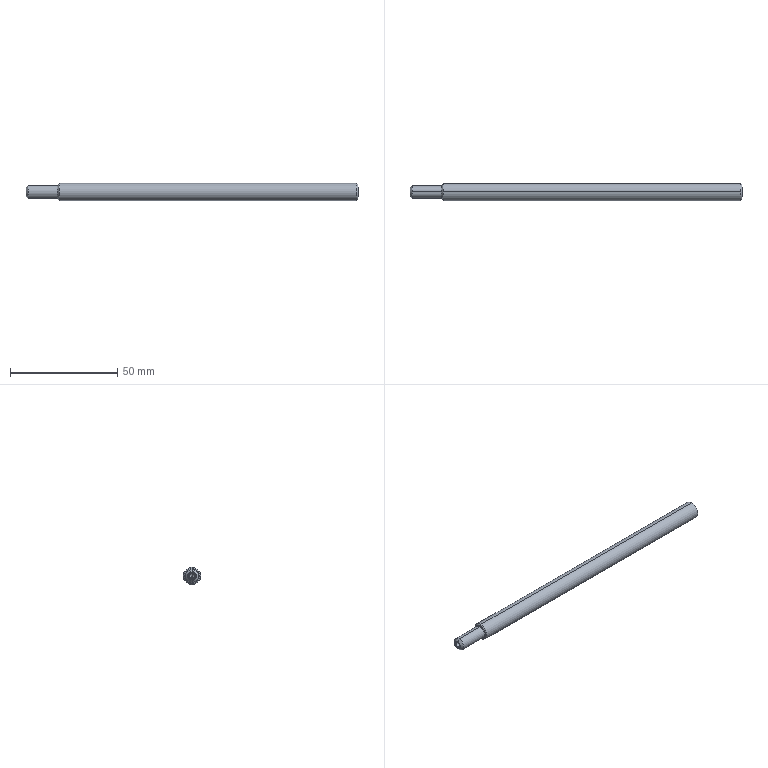Part | SolidWorks | features BaseBody 1, MoveFace 1 | 1 solid | 27 faces | box 155 x 8 x 8 mm | volume 7283 mm3 | cone 14 | cylinder 8 | plane 3 | spline 2 | commonest cylinder face diameters 2.459 x2 3.242 x2 6 x2 8 x2
STEP:
#1=CARTESIAN_POINT('',(-15.3,0.,3.));
#2=VERTEX_POINT('',#1);
#3=CARTESIAN_POINT('',(-15.3,0.,-3.));
#4=VERTEX_POINT('',#3);
#5=CARTESIAN_POINT('',(-15.3,0.,0.));
#6=DIRECTION('',(-1.,0.,0.));
#7=DIRECTION('',(0.,0.,-1.));
#8=AXIS2_PLACEMENT_3D('',#5,#6,#7);
#9=CIRCLE('',#8,3.);
#10=EDGE_CURVE('',#2,#4,#9,.T.);
#11=ORIENTED_EDGE('',*,*,#10,.F.);
#12=CARTESIAN_POINT('',(-15.,0.,3.3));
#13=VERTEX_POINT('',#12);
#14=CARTESIAN_POINT('',(-15.3,0.,3.3));
#15=DIRECTION('',(0.,-1.,0.));
#16=DIRECTION('',(0.,0.,1.));
#17=AXIS2_PLACEMENT_3D('',#14,#15,#16);
#18=CIRCLE('',#17,0.3);
#19=EDGE_CURVE('',#2,#13,#18,.T.);
#20=ORIENTED_EDGE('',*,*,#19,.T.);
#21=CARTESIAN_POINT('',(-15.,0.,-3.3));
#22=VERTEX_POINT('',#21);
#23=CARTESIAN_POINT('',(-15.,0.,3.3));
#24=CARTESIAN_POINT('',(-15.,6.6,3.3));
#25=CARTESIAN_POINT('',(-15.,6.6,-3.3));
#26=CARTESIAN_POINT('',(-15.,0.,-3.3));
#27=(BOUNDED_CURVE()B_SPLINE_CURVE(3,(#23,#24,#25,#26),.UNSPECIFIED.,.F.,.F.)B_SPLINE_CURVE_WITH_KNOTS((4,4),(0.5,1.),.UNSPECIFIED.)CURVE()GEOMETRIC_REPRESENTATION_ITEM()RATIONAL_B_SPLINE_CURVE((1.,0.3333,0.3333,1.))REPRESENTATION_ITEM(''));
#28=EDGE_CURVE('',#13,#22,#27,.T.);
#29=ORIENTED_EDGE('',*,*,#28,.T.);
#30=CARTESIAN_POINT('',(-15.3,0.,-3.3));
#31=DIRECTION('',(0.,1.,0.));
#32=DIRECTION('',(0.,0.,-1.));
#33=AXIS2_PLACEMENT_3D('',#30,#31,#32);
#34=CIRCLE('',#33,0.3);
#35=EDGE_CURVE('',#4,#22,#34,.T.);
#36=ORIENTED_EDGE('',*,*,#35,.F.);
#37=EDGE_LOOP('',(#11,#20,#29,#36));
#38=FACE_OUTER_BOUND('',#37,.T.);
#39=CARTESIAN_POINT('',(-15.3,0.,-3.));
#40=CARTESIAN_POINT('',(-15.3,6.,-3.));
#41=CARTESIAN_POINT('',(-15.3,6.,3.));
#42=CARTESIAN_POINT('',(-15.3,0.,3.));
#43=CARTESIAN_POINT('',(-15.124,0.,-3.));
#44=CARTESIAN_POINT('',(-15.124,6.,-3.));
#45=CARTESIAN_POINT('',(-15.124,6.,3.));
#46=CARTESIAN_POINT('',(-15.124,0.,3.));
#47=CARTESIAN_POINT('',(-15.,0.,-3.124));
#48=CARTESIAN_POINT('',(-15.,6.249,-3.124));
#49=CARTESIAN_POINT('',(-15.,6.249,3.124));
#50=CARTESIAN_POINT('',(-15.,0.,3.124));
#51=CARTESIAN_POINT('',(-15.,0.,-3.3));
#52=CARTESIAN_POINT('',(-15.,6.6,-3.3));
#53=CARTESIAN_POINT('',(-15.,6.6,3.3));
#54=CARTESIAN_POINT('',(-15.,0.,3.3));
#55=(BOUNDED_SURFACE()B_SPLINE_SURFACE(3,3,((#39,#40,#41,#42),(#43,#44,#45,#46),(#47,#48,#49,#50),(#51,#52,#53,#54)),.UNSPECIFIED.,.F.,.F.,.F.)B_SPLINE_SURFACE_WITH_KNOTS((4,4),(4,4),(0.,1.),(0.,1.),.UNSPECIFIED.)GEOMETRIC_REPRESENTATION_ITEM()RATIONAL_B_SPLINE_SURFACE(((1.,0.3333,0.3333,1.),(0.8047,0.2682,0.2682,0.8047),(0.8047,0.2682,0.2682,0.8047),(1.,0.3333,0.3333,1.)))REPRESENTATION_ITEM('')SURFACE());
#56=ADVANCED_FACE('',(#38),#55,.F.);
#57=CARTESIAN_POINT('',(124.5,0.,4.));
#58=VERTEX_POINT('',#57);
#59=CARTESIAN_POINT('',(124.5,0.,-4.));
#60=VERTEX_POINT('',#59);
#61=CARTESIAN_POINT('',(124.5,0.,0.));
#62=DIRECTION('',(-1.,0.,0.));
#63=DIRECTION('',(0.,0.,1.));
#64=AXIS2_PLACEMENT_3D('',#61,#62,#63);
#65=CIRCLE('',#64,4.);
#66=EDGE_CURVE('',#58,#60,#65,.T.);
#67=ORIENTED_EDGE('',*,*,#66,.T.);
#68=CARTESIAN_POINT('',(-14.5,0.,-4.));
#69=VERTEX_POINT('',#68);
#70=CARTESIAN_POINT('',(110.,0.,-4.));
#71=DIRECTION('',(-1.,0.,0.));
#72=VECTOR('',#71,1000.);
#73=LINE('',#70,#72);
#74=EDGE_CURVE('',#60,#69,#73,.T.);
#75=ORIENTED_EDGE('',*,*,#74,.T.);
#76=CARTESIAN_POINT('',(-14.5,0.,4.));
#77=VERTEX_POINT('',#76);
#78=CARTESIAN_POINT('',(-14.5,0.,0.));
#79=DIRECTION('',(1.,0.,0.));
#80=DIRECTION('',(0.,0.,1.));
#81=AXIS2_PLACEMENT_3D('',#78,#79,#80);
#82=CIRCLE('',#81,4.);
#83=EDGE_CURVE('',#69,#77,#82,.T.);
#84=ORIENTED_EDGE('',*,*,#83,.T.);
#85=CARTESIAN_POINT('',(110.,0.,4.));
#86=DIRECTION('',(-1.,0.,0.));
#87=VECTOR('',#86,1000.);
#88=LINE('',#85,#87);
#89=EDGE_CURVE('',#58,#77,#88,.T.);
#90=ORIENTED_EDGE('',*,*,#89,.F.);
#91=EDGE_LOOP('',(#67,#75,#84,#90));
#92=FACE_OUTER_BOUND('',#91,.T.);
#93=CARTESIAN_POINT('',(110.,0.,0.));
#94=DIRECTION('',(-1.,0.,0.));
#95=DIRECTION('',(0.,0.,1.));
#96=AXIS2_PLACEMENT_3D('',#93,#94,#95);
#97=CYLINDRICAL_SURFACE('',#96,4.);
#98=ADVANCED_FACE('',(#92),#97,.T.);
#99=CARTESIAN_POINT('',(-15.,0.,-3.5));
#100=VERTEX_POINT('',#99);
#101=CARTESIAN_POINT('',(-15.,0.,3.5));
#102=VERTEX_POINT('',#101);
#103=CARTESIAN_POINT('',(-15.,0.,0.));
#104=DIRECTION('',(1.,0.,0.));
#105=DIRECTION('',(0.,0.,-1.));
#106=AXIS2_PLACEMENT_3D('',#103,#104,#105);
#107=CIRCLE('',#106,3.5);
#108=EDGE_CURVE('',#100,#102,#107,.T.);
#109=ORIENTED_EDGE('',*,*,#108,.T.);
#110=CARTESIAN_POINT('',(-14.5,0.,4.));
#111=DIRECTION('',(0.7071,0.,0.7071));
#112=VECTOR('',#111,1000.);
#113=LINE('',#110,#112);
#114=EDGE_CURVE('',#102,#77,#113,.T.);
#115=ORIENTED_EDGE('',*,*,#114,.T.);
#116=ORIENTED_EDGE('',*,*,#83,.F.);
#117=CARTESIAN_POINT('',(-14.5,0.,-4.));
#118=DIRECTION('',(0.7071,0.,-0.7071));
#119=VECTOR('',#118,1000.);
#120=LINE('',#117,#119);
#121=EDGE_CURVE('',#100,#69,#120,.T.);
#122=ORIENTED_EDGE('',*,*,#121,.F.);
#123=EDGE_LOOP('',(#109,#115,#116,#122));
#124=FACE_OUTER_BOUND('',#123,.T.);
#125=CARTESIAN_POINT('',(-14.5,0.,0.));
#126=DIRECTION('',(1.,0.,0.));
#127=DIRECTION('',(0.,0.,-1.));
#128=AXIS2_PLACEMENT_3D('',#125,#126,#127);
#129=CONICAL_SURFACE('',#128,4.,0.7854);
#130=ADVANCED_FACE('',(#124),#129,.T.);
#131=CARTESIAN_POINT('',(125.,0.,3.5));
#132=VERTEX_POINT('',#131);
#133=CARTESIAN_POINT('',(125.,0.,-3.5));
#134=VERTEX_POINT('',#133);
#135=CARTESIAN_POINT('',(125.,0.,0.));
#136=DIRECTION('',(-1.,0.,0.));
#137=DIRECTION('',(0.,0.,1.));
#138=AXIS2_PLACEMENT_3D('',#135,#136,#137);
#139=CIRCLE('',#138,3.5);
#140=EDGE_CURVE('',#132,#134,#139,.T.);
#141=ORIENTED_EDGE('',*,*,#140,.T.);
#142=CARTESIAN_POINT('',(124.5,0.,-4.));
#143=DIRECTION('',(-0.7071,0.,-0.7071));
#144=VECTOR('',#143,1000.);
#145=LINE('',#142,#144);
#146=EDGE_CURVE('',#134,#60,#145,.T.);
#147=ORIENTED_EDGE('',*,*,#146,.T.);
#148=ORIENTED_EDGE('',*,*,#66,.F.);
#149=CARTESIAN_POINT('',(124.5,0.,4.));
#150=DIRECTION('',(-0.7071,0.,0.7071));
#151=VECTOR('',#150,1000.);
#152=LINE('',#149,#151);
#153=EDGE_CURVE('',#132,#58,#152,.T.);
#154=ORIENTED_EDGE('',*,*,#153,.F.);
#155=EDGE_LOOP('',(#141,#147,#148,#154));
#156=FACE_OUTER_BOUND('',#155,.T.);
#157=CARTESIAN_POINT('',(124.5,0.,0.));
#158=DIRECTION('',(-1.,0.,0.));
#159=DIRECTION('',(0.,0.,1.));
#160=AXIS2_PLACEMENT_3D('',#157,#158,#159);
#161=CONICAL_SURFACE('',#160,4.,0.7854);
#162=ADVANCED_FACE('',(#156),#161,.T.);
#163=CARTESIAN_POINT('',(124.621,0.,1.621));
#164=VERTEX_POINT('',#163);
#165=CARTESIAN_POINT('',(124.621,0.,-1.621));
#166=VERTEX_POINT('',#165);
#167=CARTESIAN_POINT('',(124.621,0.,0.));
#168=DIRECTION('',(1.,0.,0.));
#169=DIRECTION('',(0.,0.,-1.));
#170=AXIS2_PLACEMENT_3D('',#167,#168,#169);
#171=CIRCLE('',#170,1.621);
#172=EDGE_CURVE('',#164,#166,#171,.T.);
#173=ORIENTED_EDGE('',*,*,#172,.F.);
#174=CARTESIAN_POINT('',(125.,0.,2.));
#175=VERTEX_POINT('',#174);
#176=CARTESIAN_POINT('',(125.,0.,2.));
#177=DIRECTION('',(0.7071,0.,0.7071));
#178=VECTOR('',#177,1000.);
#179=LINE('',#176,#178);
#180=EDGE_CURVE('',#164,#175,#179,.T.);
#181=ORIENTED_EDGE('',*,*,#180,.T.);
#182=CARTESIAN_POINT('',(125.,0.,-2.));
#183=VERTEX_POINT('',#182);
#184=CARTESIAN_POINT('',(125.,0.,0.));
#185=DIRECTION('',(1.,0.,0.));
#186=DIRECTION('',(0.,0.,-1.));
#187=AXIS2_PLACEMENT_3D('',#184,#185,#186);
#188=CIRCLE('',#187,2.);
#189=EDGE_CURVE('',#175,#183,#188,.T.);
#190=ORIENTED_EDGE('',*,*,#189,.T.);
#191=CARTESIAN_POINT('',(125.,0.,-2.));
#192=DIRECTION('',(0.7071,0.,-0.7071));
#193=VECTOR('',#192,1000.);
#194=LINE('',#191,#193);
#195=EDGE_CURVE('',#166,#183,#194,.T.);
#196=ORIENTED_EDGE('',*,*,#195,.F.);
#197=EDGE_LOOP('',(#173,#181,#190,#196));
#198=FACE_OUTER_BOUND('',#197,.T.);
#199=CARTESIAN_POINT('',(125.,0.,0.));
#200=DIRECTION('',(1.,0.,0.));
#201=DIRECTION('',(0.,0.,-1.));
#202=AXIS2_PLACEMENT_3D('',#199,#200,#201);
#203=CONICAL_SURFACE('',#202,2.,0.7854);
#204=ADVANCED_FACE('',(#198),#203,.F.);
#205=ORIENTED_EDGE('',*,*,#10,.T.);
#206=CARTESIAN_POINT('',(-29.,0.,-3.));
#207=VERTEX_POINT('',#206);
#208=CARTESIAN_POINT('',(110.,0.,-3.));
#209=DIRECTION('',(-1.,0.,0.));
#210=VECTOR('',#209,1000.);
#211=LINE('',#208,#210);
#212=EDGE_CURVE('',#4,#207,#211,.T.);
#213=ORIENTED_EDGE('',*,*,#212,.T.);
#214=CARTESIAN_POINT('',(-29.,0.,3.));
#215=VERTEX_POINT('',#214);
#216=CARTESIAN_POINT('',(-29.,0.,0.));
#217=DIRECTION('',(1.,0.,0.));
#218=DIRECTION('',(0.,0.,1.));
#219=AXIS2_PLACEMENT_3D('',#216,#217,#218);
#220=CIRCLE('',#219,3.);
#221=EDGE_CURVE('',#207,#215,#220,.T.);
#222=ORIENTED_EDGE('',*,*,#221,.T.);
#223=CARTESIAN_POINT('',(110.,0.,3.));
#224=DIRECTION('',(-1.,0.,0.));
#225=VECTOR('',#224,1000.);
#226=LINE('',#223,#225);
#227=EDGE_CURVE('',#2,#215,#226,.T.);
#228=ORIENTED_EDGE('',*,*,#227,.F.);
#229=EDGE_LOOP('',(#205,#213,#222,#228));
#230=FACE_OUTER_BOUND('',#229,.T.);
#231=CARTESIAN_POINT('',(110.,0.,0.));
#232=DIRECTION('',(-1.,0.,0.));
#233=DIRECTION('',(0.,0.,1.));
#234=AXIS2_PLACEMENT_3D('',#231,#232,#233);
#235=CYLINDRICAL_SURFACE('',#234,3.);
#236=ADVANCED_FACE('',(#230),#235,.T.);
#237=ORIENTED_EDGE('',*,*,#172,.T.);
#238=CARTESIAN_POINT('',(111.936,0.,-1.621));
#239=VERTEX_POINT('',#238);
#240=CARTESIAN_POINT('',(125.,0.,-1.621));
#241=DIRECTION('',(-1.,0.,0.));
#242=VECTOR('',#241,1000.);
#243=LINE('',#240,#242);
#244=EDGE_CURVE('',#166,#239,#243,.T.);
#245=ORIENTED_EDGE('',*,*,#244,.T.);
#246=CARTESIAN_POINT('',(111.936,0.,1.621));
#247=VERTEX_POINT('',#246);
#248=CARTESIAN_POINT('',(111.936,0.,0.));
#249=DIRECTION('',(1.,0.,0.));
#250=DIRECTION('',(0.,0.,1.));
#251=AXIS2_PLACEMENT_3D('',#248,#249,#250);
#252=CIRCLE('',#251,1.621);
#253=EDGE_CURVE('',#247,#239,#252,.T.);
#254=ORIENTED_EDGE('',*,*,#253,.F.);
#255=CARTESIAN_POINT('',(125.,0.,1.621));
#256=DIRECTION('',(-1.,0.,0.));
#257=VECTOR('',#256,1000.);
#258=LINE('',#255,#257);
#259=EDGE_CURVE('',#164,#247,#258,.T.);
#260=ORIENTED_EDGE('',*,*,#259,.F.);
#261=EDGE_LOOP('',(#237,#245,#254,#260));
#262=FACE_OUTER_BOUND('',#261,.T.);
#263=CARTESIAN_POINT('',(125.,0.,0.));
#264=DIRECTION('',(-1.,0.,0.));
#265=DIRECTION('',(0.,0.,1.));
#266=AXIS2_PLACEMENT_3D('',#263,#264,#265);
#267=CYLINDRICAL_SURFACE('',#266,1.621);
#268=ADVANCED_FACE('',(#262),#267,.F.);
#269=CARTESIAN_POINT('',(-30.,0.,-2.));
#270=VERTEX_POINT('',#269);
#271=CARTESIAN_POINT('',(-30.,0.,2.));
#272=VERTEX_POINT('',#271);
#273=CARTESIAN_POINT('',(-30.,0.,0.));
#274=DIRECTION('',(1.,0.,0.));
#275=DIRECTION('',(0.,0.,-1.));
#276=AXIS2_PLACEMENT_3D('',#273,#274,#275);
#277=CIRCLE('',#276,2.);
#278=EDGE_CURVE('',#270,#272,#277,.T.);
#279=ORIENTED_EDGE('',*,*,#278,.T.);
#280=CARTESIAN_POINT('',(-29.,0.,3.));
#281=DIRECTION('',(0.7071,0.,0.7071));
#282=VECTOR('',#281,1000.);
#283=LINE('',#280,#282);
#284=EDGE_CURVE('',#272,#215,#283,.T.);
#285=ORIENTED_EDGE('',*,*,#284,.T.);
#286=ORIENTED_EDGE('',*,*,#221,.F.);
#287=CARTESIAN_POINT('',(-29.,0.,-3.));
#288=DIRECTION('',(0.7071,0.,-0.7071));
#289=VECTOR('',#288,1000.);
#290=LINE('',#287,#289);
#291=EDGE_CURVE('',#270,#207,#290,.T.);
#292=ORIENTED_EDGE('',*,*,#291,.F.);
#293=EDGE_LOOP('',(#279,#285,#286,#292));
#294=FACE_OUTER_BOUND('',#293,.T.);
#295=CARTESIAN_POINT('',(-29.,0.,0.));
#296=DIRECTION('',(1.,0.,0.));
#297=DIRECTION('',(0.,0.,-1.));
#298=AXIS2_PLACEMENT_3D('',#295,#296,#297);
#299=CONICAL_SURFACE('',#298,3.,0.7854);
#300=ADVANCED_FACE('',(#294),#299,.T.);
#301=CARTESIAN_POINT('',(111.,0.,0.));
#302=VERTEX_POINT('',#301);
#303=CARTESIAN_POINT('',(111.936,0.,-1.621));
#304=DIRECTION('',(0.5,0.,-0.866));
#305=VECTOR('',#304,1000.);
#306=LINE('',#303,#305);
#307=EDGE_CURVE('',#302,#239,#306,.T.);
#308=ORIENTED_EDGE('',*,*,#307,.F.);
#309=CARTESIAN_POINT('',(111.936,0.,1.621));
#310=DIRECTION('',(0.5,0.,0.866));
#311=VECTOR('',#310,1000.);
#312=LINE('',#309,#311);
#313=EDGE_CURVE('',#302,#247,#312,.T.);
#314=ORIENTED_EDGE('',*,*,#313,.T.);
#315=ORIENTED_EDGE('',*,*,#253,.T.);
#316=EDGE_LOOP('',(#308,#314,#315));
#317=FACE_OUTER_BOUND('',#316,.T.);
#318=CARTESIAN_POINT('',(111.936,0.,0.));
#319=DIRECTION('',(1.,0.,0.));
#320=DIRECTION('',(0.,0.,-1.));
#321=AXIS2_PLACEMENT_3D('',#318,#319,#320);
#322=CONICAL_SURFACE('',#321,1.621,1.047);
#323=ADVANCED_FACE('',(#317),#322,.F.);
#324=CARTESIAN_POINT('',(-29.729,0.,-1.23));
#325=VERTEX_POINT('',#324);
#326=CARTESIAN_POINT('',(-29.729,0.,1.23));
#327=VERTEX_POINT('',#326);
#328=CARTESIAN_POINT('',(-29.729,0.,0.));
#329=DIRECTION('',(-1.,0.,0.));
#330=DIRECTION('',(0.,0.,1.));
#331=AXIS2_PLACEMENT_3D('',#328,#329,#330);
#332=CIRCLE('',#331,1.23);
#333=EDGE_CURVE('',#325,#327,#332,.T.);
#334=ORIENTED_EDGE('',*,*,#333,.F.);
#335=CARTESIAN_POINT('',(-30.,0.,-1.5));
#336=VERTEX_POINT('',#335);
#337=CARTESIAN_POINT('',(-30.,0.,-1.5));
#338=DIRECTION('',(-0.7071,0.,-0.7071));
#339=VECTOR('',#338,1000.);
#340=LINE('',#337,#339);
#341=EDGE_CURVE('',#325,#336,#340,.T.);
#342=ORIENTED_EDGE('',*,*,#341,.T.);
#343=CARTESIAN_POINT('',(-30.,0.,1.5));
#344=VERTEX_POINT('',#343);
#345=CARTESIAN_POINT('',(-30.,0.,0.));
#346=DIRECTION('',(-1.,0.,0.));
#347=DIRECTION('',(0.,0.,1.));
#348=AXIS2_PLACEMENT_3D('',#345,#346,#347);
#349=CIRCLE('',#348,1.5);
#350=EDGE_CURVE('',#336,#344,#349,.T.);
#351=ORIENTED_EDGE('',*,*,#350,.T.);
#352=CARTESIAN_POINT('',(-30.,0.,1.5));
#353=DIRECTION('',(-0.7071,0.,0.7071));
#354=VECTOR('',#353,1000.);
#355=LINE('',#352,#354);
#356=EDGE_CURVE('',#327,#344,#355,.T.);
#357=ORIENTED_EDGE('',*,*,#356,.F.);
#358=EDGE_LOOP('',(#334,#342,#351,#357));
#359=FACE_OUTER_BOUND('',#358,.T.);
#360=CARTESIAN_POINT('',(-30.,0.,0.));
#361=DIRECTION('',(-1.,0.,0.));
#362=DIRECTION('',(0.,0.,1.));
#363=AXIS2_PLACEMENT_3D('',#360,#361,#362);
#364=CONICAL_SURFACE('',#363,1.5,0.7854);
#365=ADVANCED_FACE('',(#359),#364,.F.);
#366=CARTESIAN_POINT('',(-19.21,0.,-1.23));
#367=VERTEX_POINT('',#366);
#368=CARTESIAN_POINT('',(-19.21,0.,1.23));
#369=VERTEX_POINT('',#368);
#370=CARTESIAN_POINT('',(-19.21,0.,0.));
#371=DIRECTION('',(-1.,0.,0.));
#372=DIRECTION('',(0.,0.,1.));
#373=AXIS2_PLACEMENT_3D('',#370,#371,#372);
#374=CIRCLE('',#373,1.23);
#375=EDGE_CURVE('',#367,#369,#374,.T.);
#376=ORIENTED_EDGE('',*,*,#375,.F.);
#377=CARTESIAN_POINT('',(-18.5,0.,-1.23));
#378=DIRECTION('',(-1.,0.,0.));
#379=VECTOR('',#378,1000.);
#380=LINE('',#377,#379);
#381=EDGE_CURVE('',#367,#325,#380,.T.);
#382=ORIENTED_EDGE('',*,*,#381,.T.);
#383=ORIENTED_EDGE('',*,*,#333,.T.);
#384=CARTESIAN_POINT('',(-18.5,0.,1.23));
#385=DIRECTION('',(-1.,0.,0.));
#386=VECTOR('',#385,1000.);
#387=LINE('',#384,#386);
#388=EDGE_CURVE('',#369,#327,#387,.T.);
#389=ORIENTED_EDGE('',*,*,#388,.F.);
#390=EDGE_LOOP('',(#376,#382,#383,#389));
#391=FACE_OUTER_BOUND('',#390,.T.);
#392=CARTESIAN_POINT('',(-18.5,0.,0.));
#393=DIRECTION('',(-1.,0.,0.));
#394=DIRECTION('',(0.,0.,1.));
#395=AXIS2_PLACEMENT_3D('',#392,#393,#394);
#396=CYLINDRICAL_SURFACE('',#395,1.23);
#397=ADVANCED_FACE('',(#391),#396,.F.);
#398=CARTESIAN_POINT('',(-18.5,0.,0.));
#399=VERTEX_POINT('',#398);
#400=CARTESIAN_POINT('',(-19.21,0.,1.23));
#401=DIRECTION('',(-0.5,0.,0.866));
#402=VECTOR('',#401,1000.);
#403=LINE('',#400,#402);
#404=EDGE_CURVE('',#399,#369,#403,.T.);
#405=ORIENTED_EDGE('',*,*,#404,.F.);
#406=CARTESIAN_POINT('',(-19.21,0.,-1.23));
#407=DIRECTION('',(-0.5,0.,-0.866));
#408=VECTOR('',#407,1000.);
#409=LINE('',#406,#408);
#410=EDGE_CURVE('',#399,#367,#409,.T.);
#411=ORIENTED_EDGE('',*,*,#410,.T.);
#412=ORIENTED_EDGE('',*,*,#375,.T.);
#413=EDGE_LOOP('',(#405,#411,#412));
#414=FACE_OUTER_BOUND('',#413,.T.);
#415=CARTESIAN_POINT('',(-19.21,0.,0.));
#416=DIRECTION('',(-1.,0.,0.));
#417=DIRECTION('',(0.,0.,1.));
#418=AXIS2_PLACEMENT_3D('',#415,#416,#417);
#419=CONICAL_SURFACE('',#418,1.23,1.047);
#420=ADVANCED_FACE('',(#414),#419,.F.);
#421=ORIENTED_EDGE('',*,*,#74,.F.);
#422=CARTESIAN_POINT('',(124.5,0.,0.));
#423=DIRECTION('',(-1.,0.,0.));
#424=DIRECTION('',(0.,0.,1.));
#425=AXIS2_PLACEMENT_3D('',#422,#423,#424);
#426=CIRCLE('',#425,4.);
#427=EDGE_CURVE('',#60,#58,#426,.T.);
#428=ORIENTED_EDGE('',*,*,#427,.T.);
#429=ORIENTED_EDGE('',*,*,#89,.T.);
#430=CARTESIAN_POINT('',(-14.5,0.,0.));
#431=DIRECTION('',(1.,0.,0.));
#432=DIRECTION('',(0.,0.,1.));
#433=AXIS2_PLACEMENT_3D('',#430,#431,#432);
#434=CIRCLE('',#433,4.);
#435=EDGE_CURVE('',#77,#69,#434,.T.);
#436=ORIENTED_EDGE('',*,*,#435,.T.);
#437=EDGE_LOOP('',(#421,#428,#429,#436));
#438=FACE_OUTER_BOUND('',#437,.T.);
#439=CARTESIAN_POINT('',(110.,0.,0.));
#440=DIRECTION('',(-1.,0.,0.));
#441=DIRECTION('',(0.,0.,1.));
#442=AXIS2_PLACEMENT_3D('',#439,#440,#441);
#443=CYLINDRICAL_SURFACE('',#442,4.);
#444=ADVANCED_FACE('',(#438),#443,.T.);
#445=ORIENTED_EDGE('',*,*,#114,.F.);
#446=CARTESIAN_POINT('',(-15.,0.,0.));
#447=DIRECTION('',(1.,0.,0.));
#448=DIRECTION('',(0.,0.,-1.));
#449=AXIS2_PLACEMENT_3D('',#446,#447,#448);
#450=CIRCLE('',#449,3.5);
#451=EDGE_CURVE('',#102,#100,#450,.T.);
#452=ORIENTED_EDGE('',*,*,#451,.T.);
#453=ORIENTED_EDGE('',*,*,#121,.T.);
#454=ORIENTED_EDGE('',*,*,#435,.F.);
#455=EDGE_LOOP('',(#445,#452,#453,#454));
#456=FACE_OUTER_BOUND('',#455,.T.);
#457=CARTESIAN_POINT('',(-14.5,0.,0.));
#458=DIRECTION('',(1.,0.,0.));
#459=DIRECTION('',(0.,0.,-1.));
#460=AXIS2_PLACEMENT_3D('',#457,#458,#459);
#461=CONICAL_SURFACE('',#460,4.,0.7854);
#462=ADVANCED_FACE('',(#456),#461,.T.);
#463=ORIENTED_EDGE('',*,*,#146,.F.);
#464=CARTESIAN_POINT('',(125.,0.,0.));
#465=DIRECTION('',(-1.,0.,0.));
#466=DIRECTION('',(0.,0.,1.));
#467=AXIS2_PLACEMENT_3D('',#464,#465,#466);
#468=CIRCLE('',#467,3.5);
#469=EDGE_CURVE('',#134,#132,#468,.T.);
#470=ORIENTED_EDGE('',*,*,#469,.T.);
#471=ORIENTED_EDGE('',*,*,#153,.T.);
#472=ORIENTED_EDGE('',*,*,#427,.F.);
#473=EDGE_LOOP('',(#463,#470,#471,#472));
#474=FACE_OUTER_BOUND('',#473,.T.);
#475=CARTESIAN_POINT('',(124.5,0.,0.));
#476=DIRECTION('',(-1.,0.,0.));
#477=DIRECTION('',(0.,0.,1.));
#478=AXIS2_PLACEMENT_3D('',#475,#476,#477);
#479=CONICAL_SURFACE('',#478,4.,0.7854);
#480=ADVANCED_FACE('',(#474),#479,.T.);
#481=CARTESIAN_POINT('',(-15.,0.,-3.3));
#482=CARTESIAN_POINT('',(-15.,-6.6,-3.3));
#483=CARTESIAN_POINT('',(-15.,-6.6,3.3));
#484=CARTESIAN_POINT('',(-15.,0.,3.3));
#485=(BOUNDED_CURVE()B_SPLINE_CURVE(3,(#481,#482,#483,#484),.UNSPECIFIED.,.F.,.F.)B_SPLINE_CURVE_WITH_KNOTS((4,4),(0.,0.5),.UNSPECIFIED.)CURVE()GEOMETRIC_REPRESENTATION_ITEM()RATIONAL_B_SPLINE_CURVE((1.,0.3333,0.3333,1.))REPRESENTATION_ITEM(''));
#486=EDGE_CURVE('',#22,#13,#485,.T.);
#487=ORIENTED_EDGE('',*,*,#486,.F.);
#488=ORIENTED_EDGE('',*,*,#28,.F.);
#489=EDGE_LOOP('',(#487,#488));
#490=FACE_BOUND('',#489,.T.);
#491=ORIENTED_EDGE('',*,*,#108,.F.);
#492=ORIENTED_EDGE('',*,*,#451,.F.);
#493=EDGE_LOOP('',(#491,#492));
#494=FACE_OUTER_BOUND('',#493,.T.);
#495=CARTESIAN_POINT('',(-15.,3.3,0.));
#496=DIRECTION('',(1.,0.,0.));
#497=DIRECTION('',(0.,0.,-1.));
#498=AXIS2_PLACEMENT_3D('',#495,#496,#497);
#499=PLANE('',#498);
#500=ADVANCED_FACE('',(#490,#494),#499,.F.);
#501=ORIENTED_EDGE('',*,*,#140,.F.);
#502=ORIENTED_EDGE('',*,*,#469,.F.);
#503=EDGE_LOOP('',(#501,#502));
#504=FACE_OUTER_BOUND('',#503,.T.);
#505=CARTESIAN_POINT('',(125.,0.,0.));
#506=DIRECTION('',(1.,0.,0.));
#507=DIRECTION('',(0.,0.,-1.));
#508=AXIS2_PLACEMENT_3D('',#505,#506,#507);
#509=CIRCLE('',#508,2.);
#510=EDGE_CURVE('',#183,#175,#509,.T.);
#511=ORIENTED_EDGE('',*,*,#510,.F.);
#512=ORIENTED_EDGE('',*,*,#189,.F.);
#513=EDGE_LOOP('',(#511,#512));
#514=FACE_BOUND('',#513,.T.);
#515=CARTESIAN_POINT('',(125.,3.5,0.));
#516=DIRECTION('',(-1.,0.,0.));
#517=DIRECTION('',(0.,0.,1.));
#518=AXIS2_PLACEMENT_3D('',#515,#516,#517);
#519=PLANE('',#518);
#520=ADVANCED_FACE('',(#504,#514),#519,.F.);
#521=ORIENTED_EDGE('',*,*,#19,.F.);
#522=CARTESIAN_POINT('',(-15.3,0.,0.));
#523=DIRECTION('',(-1.,0.,0.));
#524=DIRECTION('',(0.,0.,-1.));
#525=AXIS2_PLACEMENT_3D('',#522,#523,#524);
#526=CIRCLE('',#525,3.);
#527=EDGE_CURVE('',#4,#2,#526,.T.);
#528=ORIENTED_EDGE('',*,*,#527,.F.);
#529=ORIENTED_EDGE('',*,*,#35,.T.);
#530=ORIENTED_EDGE('',*,*,#486,.T.);
#531=EDGE_LOOP('',(#521,#528,#529,#530));
#532=FACE_OUTER_BOUND('',#531,.T.);
#533=CARTESIAN_POINT('',(-15.3,0.,3.));
#534=CARTESIAN_POINT('',(-15.3,-6.,3.));
#535=CARTESIAN_POINT('',(-15.3,-6.,-3.));
#536=CARTESIAN_POINT('',(-15.3,0.,-3.));
#537=CARTESIAN_POINT('',(-15.124,0.,3.));
#538=CARTESIAN_POINT('',(-15.124,-6.,3.));
#539=CARTESIAN_POINT('',(-15.124,-6.,-3.));
#540=CARTESIAN_POINT('',(-15.124,0.,-3.));
#541=CARTESIAN_POINT('',(-15.,0.,3.124));
#542=CARTESIAN_POINT('',(-15.,-6.249,3.124));
#543=CARTESIAN_POINT('',(-15.,-6.249,-3.124));
#544=CARTESIAN_POINT('',(-15.,0.,-3.124));
#545=CARTESIAN_POINT('',(-15.,0.,3.3));
#546=CARTESIAN_POINT('',(-15.,-6.6,3.3));
#547=CARTESIAN_POINT('',(-15.,-6.6,-3.3));
#548=CARTESIAN_POINT('',(-15.,0.,-3.3));
#549=(BOUNDED_SURFACE()B_SPLINE_SURFACE(3,3,((#533,#534,#535,#536),(#537,#538,#539,#540),(#541,#542,#543,#544),(#545,#546,#547,#548)),.UNSPECIFIED.,.F.,.F.,.T.)B_SPLINE_SURFACE_WITH_KNOTS((4,4),(4,4),(0.,1.),(0.,1.),.UNSPECIFIED.)GEOMETRIC_REPRESENTATION_ITEM()RATIONAL_B_SPLINE_SURFACE(((1.,0.3333,0.3333,1.),(0.8047,0.2682,0.2682,0.8047),(0.8047,0.2682,0.2682,0.8047),(1.,0.3333,0.3333,1.)))REPRESENTATION_ITEM('')SURFACE());
#550=ADVANCED_FACE('',(#532),#549,.F.);
#551=ORIENTED_EDGE('',*,*,#180,.F.);
#552=CARTESIAN_POINT('',(124.621,0.,0.));
#553=DIRECTION('',(1.,0.,0.));
#554=DIRECTION('',(0.,0.,-1.));
#555=AXIS2_PLACEMENT_3D('',#552,#553,#554);
#556=CIRCLE('',#555,1.621);
#557=EDGE_CURVE('',#166,#164,#556,.T.);
#558=ORIENTED_EDGE('',*,*,#557,.F.);
#559=ORIENTED_EDGE('',*,*,#195,.T.);
#560=ORIENTED_EDGE('',*,*,#510,.T.);
#561=EDGE_LOOP('',(#551,#558,#559,#560));
#562=FACE_OUTER_BOUND('',#561,.T.);
#563=CARTESIAN_POINT('',(125.,0.,0.));
#564=DIRECTION('',(1.,0.,0.));
#565=DIRECTION('',(0.,0.,-1.));
#566=AXIS2_PLACEMENT_3D('',#563,#564,#565);
#567=CONICAL_SURFACE('',#566,2.,0.7854);
#568=ADVANCED_FACE('',(#562),#567,.F.);
#569=ORIENTED_EDGE('',*,*,#212,.F.);
#570=ORIENTED_EDGE('',*,*,#527,.T.);
#571=ORIENTED_EDGE('',*,*,#227,.T.);
#572=CARTESIAN_POINT('',(-29.,0.,0.));
#573=DIRECTION('',(1.,0.,0.));
#574=DIRECTION('',(0.,0.,1.));
#575=AXIS2_PLACEMENT_3D('',#572,#573,#574);
#576=CIRCLE('',#575,3.);
#577=EDGE_CURVE('',#215,#207,#576,.T.);
#578=ORIENTED_EDGE('',*,*,#577,.T.);
#579=EDGE_LOOP('',(#569,#570,#571,#578));
#580=FACE_OUTER_BOUND('',#579,.T.);
#581=CARTESIAN_POINT('',(110.,0.,0.));
#582=DIRECTION('',(-1.,0.,0.));
#583=DIRECTION('',(0.,0.,1.));
#584=AXIS2_PLACEMENT_3D('',#581,#582,#583);
#585=CYLINDRICAL_SURFACE('',#584,3.);
#586=ADVANCED_FACE('',(#580),#585,.T.);
#587=ORIENTED_EDGE('',*,*,#244,.F.);
#588=ORIENTED_EDGE('',*,*,#557,.T.);
#589=ORIENTED_EDGE('',*,*,#259,.T.);
#590=CARTESIAN_POINT('',(111.936,0.,0.));
#591=DIRECTION('',(1.,0.,0.));
#592=DIRECTION('',(0.,0.,1.));
#593=AXIS2_PLACEMENT_3D('',#590,#591,#592);
#594=CIRCLE('',#593,1.621);
#595=EDGE_CURVE('',#239,#247,#594,.T.);
#596=ORIENTED_EDGE('',*,*,#595,.F.);
#597=EDGE_LOOP('',(#587,#588,#589,#596));
#598=FACE_OUTER_BOUND('',#597,.T.);
#599=CARTESIAN_POINT('',(125.,0.,0.));
#600=DIRECTION('',(-1.,0.,0.));
#601=DIRECTION('',(0.,0.,1.));
#602=AXIS2_PLACEMENT_3D('',#599,#600,#601);
#603=CYLINDRICAL_SURFACE('',#602,1.621);
#604=ADVANCED_FACE('',(#598),#603,.F.);
#605=ORIENTED_EDGE('',*,*,#284,.F.);
#606=CARTESIAN_POINT('',(-30.,0.,0.));
#607=DIRECTION('',(1.,0.,0.));
#608=DIRECTION('',(0.,0.,-1.));
#609=AXIS2_PLACEMENT_3D('',#606,#607,#608);
#610=CIRCLE('',#609,2.);
#611=EDGE_CURVE('',#272,#270,#610,.T.);
#612=ORIENTED_EDGE('',*,*,#611,.T.);
#613=ORIENTED_EDGE('',*,*,#291,.T.);
#614=ORIENTED_EDGE('',*,*,#577,.F.);
#615=EDGE_LOOP('',(#605,#612,#613,#614));
#616=FACE_OUTER_BOUND('',#615,.T.);
#617=CARTESIAN_POINT('',(-29.,0.,0.));
#618=DIRECTION('',(1.,0.,0.));
#619=DIRECTION('',(0.,0.,-1.));
#620=AXIS2_PLACEMENT_3D('',#617,#618,#619);
#621=CONICAL_SURFACE('',#620,3.,0.7854);
#622=ADVANCED_FACE('',(#616),#621,.T.);
#623=ORIENTED_EDGE('',*,*,#313,.F.);
#624=ORIENTED_EDGE('',*,*,#307,.T.);
#625=ORIENTED_EDGE('',*,*,#595,.T.);
#626=EDGE_LOOP('',(#623,#624,#625));
#627=FACE_OUTER_BOUND('',#626,.T.);
#628=CARTESIAN_POINT('',(111.936,0.,0.));
#629=DIRECTION('',(1.,0.,0.));
#630=DIRECTION('',(0.,0.,-1.));
#631=AXIS2_PLACEMENT_3D('',#628,#629,#630);
#632=CONICAL_SURFACE('',#631,1.621,1.047);
#633=ADVANCED_FACE('',(#627),#632,.F.);
#634=CARTESIAN_POINT('',(-30.,0.,0.));
#635=DIRECTION('',(-1.,0.,0.));
#636=DIRECTION('',(0.,0.,1.));
#637=AXIS2_PLACEMENT_3D('',#634,#635,#636);
#638=CIRCLE('',#637,1.5);
#639=EDGE_CURVE('',#344,#336,#638,.T.);
#640=ORIENTED_EDGE('',*,*,#639,.F.);
#641=ORIENTED_EDGE('',*,*,#350,.F.);
#642=EDGE_LOOP('',(#640,#641));
#643=FACE_BOUND('',#642,.T.);
#644=ORIENTED_EDGE('',*,*,#278,.F.);
#645=ORIENTED_EDGE('',*,*,#611,.F.);
#646=EDGE_LOOP('',(#644,#645));
#647=FACE_OUTER_BOUND('',#646,.T.);
#648=CARTESIAN_POINT('',(-30.,0.,0.));
#649=DIRECTION('',(1.,0.,0.));
#650=DIRECTION('',(0.,0.,-1.));
#651=AXIS2_PLACEMENT_3D('',#648,#649,#650);
#652=PLANE('',#651);
#653=ADVANCED_FACE('',(#643,#647),#652,.F.);
#654=ORIENTED_EDGE('',*,*,#341,.F.);
#655=CARTESIAN_POINT('',(-29.729,0.,0.));
#656=DIRECTION('',(-1.,0.,0.));
#657=DIRECTION('',(0.,0.,1.));
#658=AXIS2_PLACEMENT_3D('',#655,#656,#657);
#659=CIRCLE('',#658,1.23);
#660=EDGE_CURVE('',#327,#325,#659,.T.);
#661=ORIENTED_EDGE('',*,*,#660,.F.);
#662=ORIENTED_EDGE('',*,*,#356,.T.);
#663=ORIENTED_EDGE('',*,*,#639,.T.);
#664=EDGE_LOOP('',(#654,#661,#662,#663));
#665=FACE_OUTER_BOUND('',#664,.T.);
#666=CARTESIAN_POINT('',(-30.,0.,0.));
#667=DIRECTION('',(-1.,0.,0.));
#668=DIRECTION('',(0.,0.,1.));
#669=AXIS2_PLACEMENT_3D('',#666,#667,#668);
#670=CONICAL_SURFACE('',#669,1.5,0.7854);
#671=ADVANCED_FACE('',(#665),#670,.F.);
#672=ORIENTED_EDGE('',*,*,#381,.F.);
#673=CARTESIAN_POINT('',(-19.21,0.,0.));
#674=DIRECTION('',(-1.,0.,0.));
#675=DIRECTION('',(0.,0.,1.));
#676=AXIS2_PLACEMENT_3D('',#673,#674,#675);
#677=CIRCLE('',#676,1.23);
#678=EDGE_CURVE('',#369,#367,#677,.T.);
#679=ORIENTED_EDGE('',*,*,#678,.F.);
#680=ORIENTED_EDGE('',*,*,#388,.T.);
#681=ORIENTED_EDGE('',*,*,#660,.T.);
#682=EDGE_LOOP('',(#672,#679,#680,#681));
#683=FACE_OUTER_BOUND('',#682,.T.);
#684=CARTESIAN_POINT('',(-18.5,0.,0.));
#685=DIRECTION('',(-1.,0.,0.));
#686=DIRECTION('',(0.,0.,1.));
#687=AXIS2_PLACEMENT_3D('',#684,#685,#686);
#688=CYLINDRICAL_SURFACE('',#687,1.23);
#689=ADVANCED_FACE('',(#683),#688,.F.);
#690=ORIENTED_EDGE('',*,*,#410,.F.);
#691=ORIENTED_EDGE('',*,*,#404,.T.);
#692=ORIENTED_EDGE('',*,*,#678,.T.);
#693=EDGE_LOOP('',(#690,#691,#692));
#694=FACE_OUTER_BOUND('',#693,.T.);
#695=CARTESIAN_POINT('',(-19.21,0.,0.));
#696=DIRECTION('',(-1.,0.,0.));
#697=DIRECTION('',(0.,0.,1.));
#698=AXIS2_PLACEMENT_3D('',#695,#696,#697);
#699=CONICAL_SURFACE('',#698,1.23,1.047);
#700=ADVANCED_FACE('',(#694),#699,.F.);
#701=CLOSED_SHELL('',(#56,#98,#130,#162,#204,#236,#268,#300,#323,#365,#397,#420,#444,#462,#480,#500,#520,#550,#568,#586,#604,#622,#633,#653,#671,#689,#700));
#702=MANIFOLD_SOLID_BREP('',#701);
#703=CARTESIAN_POINT('',(0.,0.,0.));
#704=DIRECTION('',(0.,0.,1.));
#705=DIRECTION('',(1.,0.,0.));
#706=AXIS2_PLACEMENT_3D('',#703,#704,#705);
#707=(LENGTH_UNIT()NAMED_UNIT(*)SI_UNIT(.MILLI.,.METRE.));
#708=UNCERTAINTY_MEASURE_WITH_UNIT(LENGTH_MEASURE(0.00001),#707,'','');
#709=(NAMED_UNIT(*)PLANE_ANGLE_UNIT()SI_UNIT($,.RADIAN.));
#710=(NAMED_UNIT(*)SI_UNIT($,.STERADIAN.)SOLID_ANGLE_UNIT());
#711=(GEOMETRIC_REPRESENTATION_CONTEXT(3)GLOBAL_UNCERTAINTY_ASSIGNED_CONTEXT((#708))GLOBAL_UNIT_ASSIGNED_CONTEXT((#707,#709,#710))REPRESENTATION_CONTEXT('',''));
#712=ADVANCED_BREP_SHAPE_REPRESENTATION('',(#702,#706),#711);